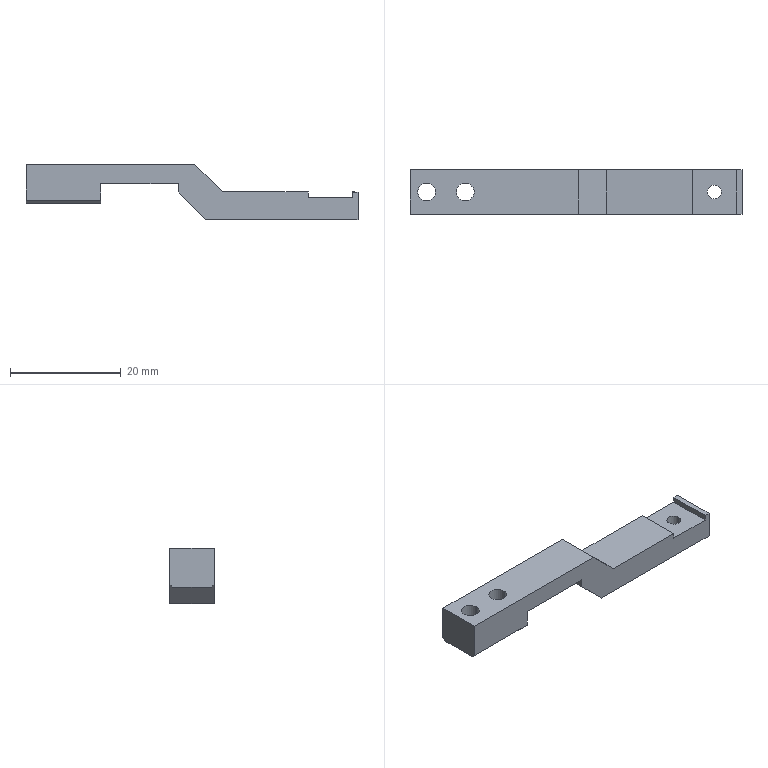Part | SolidWorks | features ICE 4, Chamfer 2, HoleWzd 2, Extrusion 1 | 1 solid | 25 faces | box 60 x 8 x 10 mm | volume 2368 mm3 | plane 19 | cylinder 6 | commonest cylinder face diameters 3.2 x4 2.5 x2
STEP:
#1=CARTESIAN_POINT('',(23.75,0.,-6.5));
#2=VERTEX_POINT('',#1);
#3=CARTESIAN_POINT('',(26.25,0.,-6.5));
#4=VERTEX_POINT('',#3);
#5=CARTESIAN_POINT('',(25.,0.,-6.5));
#6=DIRECTION('',(0.,0.,1.));
#7=DIRECTION('',(1.,0.,0.));
#8=AXIS2_PLACEMENT_3D('',#5,#6,#7);
#9=CIRCLE('',#8,1.25);
#10=EDGE_CURVE('',#2,#4,#9,.T.);
#11=ORIENTED_EDGE('',*,*,#10,.F.);
#12=CARTESIAN_POINT('',(23.75,0.,-2.5));
#13=VERTEX_POINT('',#12);
#14=CARTESIAN_POINT('',(23.75,0.,-2.5));
#15=DIRECTION('',(0.,0.,1.));
#16=VECTOR('',#15,1000.);
#17=LINE('',#14,#16);
#18=EDGE_CURVE('',#2,#13,#17,.T.);
#19=ORIENTED_EDGE('',*,*,#18,.T.);
#20=CARTESIAN_POINT('',(26.25,0.,-2.5));
#21=VERTEX_POINT('',#20);
#22=CARTESIAN_POINT('',(25.,0.,-2.5));
#23=DIRECTION('',(0.,0.,1.));
#24=DIRECTION('',(1.,0.,0.));
#25=AXIS2_PLACEMENT_3D('',#22,#23,#24);
#26=CIRCLE('',#25,1.25);
#27=EDGE_CURVE('',#13,#21,#26,.T.);
#28=ORIENTED_EDGE('',*,*,#27,.T.);
#29=CARTESIAN_POINT('',(26.25,0.,-2.5));
#30=DIRECTION('',(0.,0.,1.));
#31=VECTOR('',#30,1000.);
#32=LINE('',#29,#31);
#33=EDGE_CURVE('',#4,#21,#32,.T.);
#34=ORIENTED_EDGE('',*,*,#33,.F.);
#35=EDGE_LOOP('',(#11,#19,#28,#34));
#36=FACE_OUTER_BOUND('',#35,.T.);
#37=CARTESIAN_POINT('',(25.,0.,-2.5));
#38=DIRECTION('',(0.,0.,1.));
#39=DIRECTION('',(1.,0.,0.));
#40=AXIS2_PLACEMENT_3D('',#37,#38,#39);
#41=CYLINDRICAL_SURFACE('',#40,1.25);
#42=ADVANCED_FACE('',(#36),#41,.F.);
#43=CARTESIAN_POINT('',(-28.6,0.,-3.5));
#44=VERTEX_POINT('',#43);
#45=CARTESIAN_POINT('',(-25.4,0.,-3.5));
#46=VERTEX_POINT('',#45);
#47=CARTESIAN_POINT('',(-27.,0.,-3.5));
#48=DIRECTION('',(0.,0.,1.));
#49=DIRECTION('',(1.,0.,0.));
#50=AXIS2_PLACEMENT_3D('',#47,#48,#49);
#51=CIRCLE('',#50,1.6);
#52=EDGE_CURVE('',#44,#46,#51,.T.);
#53=ORIENTED_EDGE('',*,*,#52,.F.);
#54=CARTESIAN_POINT('',(-28.6,0.,3.5));
#55=VERTEX_POINT('',#54);
#56=CARTESIAN_POINT('',(-28.6,0.,3.5));
#57=DIRECTION('',(0.,0.,1.));
#58=VECTOR('',#57,1000.);
#59=LINE('',#56,#58);
#60=EDGE_CURVE('',#44,#55,#59,.T.);
#61=ORIENTED_EDGE('',*,*,#60,.T.);
#62=CARTESIAN_POINT('',(-25.4,0.,3.5));
#63=VERTEX_POINT('',#62);
#64=CARTESIAN_POINT('',(-27.,0.,3.5));
#65=DIRECTION('',(0.,0.,1.));
#66=DIRECTION('',(1.,0.,0.));
#67=AXIS2_PLACEMENT_3D('',#64,#65,#66);
#68=CIRCLE('',#67,1.6);
#69=EDGE_CURVE('',#55,#63,#68,.T.);
#70=ORIENTED_EDGE('',*,*,#69,.T.);
#71=CARTESIAN_POINT('',(-25.4,0.,3.5));
#72=DIRECTION('',(0.,0.,1.));
#73=VECTOR('',#72,1000.);
#74=LINE('',#71,#73);
#75=EDGE_CURVE('',#46,#63,#74,.T.);
#76=ORIENTED_EDGE('',*,*,#75,.F.);
#77=EDGE_LOOP('',(#53,#61,#70,#76));
#78=FACE_OUTER_BOUND('',#77,.T.);
#79=CARTESIAN_POINT('',(-27.,0.,3.5));
#80=DIRECTION('',(0.,0.,1.));
#81=DIRECTION('',(1.,0.,0.));
#82=AXIS2_PLACEMENT_3D('',#79,#80,#81);
#83=CYLINDRICAL_SURFACE('',#82,1.6);
#84=ADVANCED_FACE('',(#78),#83,.F.);
#85=CARTESIAN_POINT('',(-21.6,0.,-3.5));
#86=VERTEX_POINT('',#85);
#87=CARTESIAN_POINT('',(-18.4,0.,-3.5));
#88=VERTEX_POINT('',#87);
#89=CARTESIAN_POINT('',(-20.,0.,-3.5));
#90=DIRECTION('',(0.,0.,1.));
#91=DIRECTION('',(1.,0.,0.));
#92=AXIS2_PLACEMENT_3D('',#89,#90,#91);
#93=CIRCLE('',#92,1.6);
#94=EDGE_CURVE('',#86,#88,#93,.T.);
#95=ORIENTED_EDGE('',*,*,#94,.F.);
#96=CARTESIAN_POINT('',(-21.6,0.,3.5));
#97=VERTEX_POINT('',#96);
#98=CARTESIAN_POINT('',(-21.6,0.,3.5));
#99=DIRECTION('',(0.,0.,1.));
#100=VECTOR('',#99,1000.);
#101=LINE('',#98,#100);
#102=EDGE_CURVE('',#86,#97,#101,.T.);
#103=ORIENTED_EDGE('',*,*,#102,.T.);
#104=CARTESIAN_POINT('',(-18.4,0.,3.5));
#105=VERTEX_POINT('',#104);
#106=CARTESIAN_POINT('',(-20.,0.,3.5));
#107=DIRECTION('',(0.,0.,1.));
#108=DIRECTION('',(1.,0.,0.));
#109=AXIS2_PLACEMENT_3D('',#106,#107,#108);
#110=CIRCLE('',#109,1.6);
#111=EDGE_CURVE('',#97,#105,#110,.T.);
#112=ORIENTED_EDGE('',*,*,#111,.T.);
#113=CARTESIAN_POINT('',(-18.4,0.,3.5));
#114=DIRECTION('',(0.,0.,1.));
#115=VECTOR('',#114,1000.);
#116=LINE('',#113,#115);
#117=EDGE_CURVE('',#88,#105,#116,.T.);
#118=ORIENTED_EDGE('',*,*,#117,.F.);
#119=EDGE_LOOP('',(#95,#103,#112,#118));
#120=FACE_OUTER_BOUND('',#119,.T.);
#121=CARTESIAN_POINT('',(-20.,0.,3.5));
#122=DIRECTION('',(0.,0.,1.));
#123=DIRECTION('',(1.,0.,0.));
#124=AXIS2_PLACEMENT_3D('',#121,#122,#123);
#125=CYLINDRICAL_SURFACE('',#124,1.6);
#126=ADVANCED_FACE('',(#120),#125,.F.);
#127=CARTESIAN_POINT('',(21.,-4.,-1.5));
#128=VERTEX_POINT('',#127);
#129=CARTESIAN_POINT('',(5.5,-4.,-1.5));
#130=VERTEX_POINT('',#129);
#131=CARTESIAN_POINT('',(30.,-4.,-1.5));
#132=DIRECTION('',(-1.,0.,0.));
#133=VECTOR('',#132,1000.);
#134=LINE('',#131,#133);
#135=EDGE_CURVE('',#128,#130,#134,.T.);
#136=ORIENTED_EDGE('',*,*,#135,.F.);
#137=CARTESIAN_POINT('',(21.,4.,-1.5));
#138=VERTEX_POINT('',#137);
#139=CARTESIAN_POINT('',(21.,-4.,-1.5));
#140=DIRECTION('',(0.,-1.,0.));
#141=VECTOR('',#140,1000.);
#142=LINE('',#139,#141);
#143=EDGE_CURVE('',#138,#128,#142,.T.);
#144=ORIENTED_EDGE('',*,*,#143,.F.);
#145=CARTESIAN_POINT('',(5.5,4.,-1.5));
#146=VERTEX_POINT('',#145);
#147=CARTESIAN_POINT('',(30.,4.,-1.5));
#148=DIRECTION('',(-1.,0.,0.));
#149=VECTOR('',#148,1000.);
#150=LINE('',#147,#149);
#151=EDGE_CURVE('',#138,#146,#150,.T.);
#152=ORIENTED_EDGE('',*,*,#151,.T.);
#153=CARTESIAN_POINT('',(5.5,-4.,-1.5));
#154=DIRECTION('',(0.,1.,0.));
#155=VECTOR('',#154,1000.);
#156=LINE('',#153,#155);
#157=EDGE_CURVE('',#130,#146,#156,.T.);
#158=ORIENTED_EDGE('',*,*,#157,.F.);
#159=EDGE_LOOP('',(#136,#144,#152,#158));
#160=FACE_OUTER_BOUND('',#159,.T.);
#161=CARTESIAN_POINT('',(30.,-4.,-1.5));
#162=DIRECTION('',(0.,0.,-1.));
#163=DIRECTION('',(-1.,0.,0.));
#164=AXIS2_PLACEMENT_3D('',#161,#162,#163);
#165=PLANE('',#164);
#166=ADVANCED_FACE('',(#160),#165,.F.);
#167=CARTESIAN_POINT('',(-27.,0.,-3.5));
#168=DIRECTION('',(0.,0.,1.));
#169=DIRECTION('',(1.,0.,0.));
#170=AXIS2_PLACEMENT_3D('',#167,#168,#169);
#171=CIRCLE('',#170,1.6);
#172=EDGE_CURVE('',#46,#44,#171,.T.);
#173=ORIENTED_EDGE('',*,*,#172,.T.);
#174=ORIENTED_EDGE('',*,*,#52,.T.);
#175=EDGE_LOOP('',(#173,#174));
#176=FACE_BOUND('',#175,.T.);
#177=CARTESIAN_POINT('',(-20.,0.,-3.5));
#178=DIRECTION('',(0.,0.,1.));
#179=DIRECTION('',(1.,0.,0.));
#180=AXIS2_PLACEMENT_3D('',#177,#178,#179);
#181=CIRCLE('',#180,1.6);
#182=EDGE_CURVE('',#88,#86,#181,.T.);
#183=ORIENTED_EDGE('',*,*,#182,.T.);
#184=ORIENTED_EDGE('',*,*,#94,.T.);
#185=EDGE_LOOP('',(#183,#184));
#186=FACE_BOUND('',#185,.T.);
#187=CARTESIAN_POINT('',(-16.5,-3.5,-3.5));
#188=VERTEX_POINT('',#187);
#189=CARTESIAN_POINT('',(-16.5,3.5,-3.5));
#190=VERTEX_POINT('',#189);
#191=CARTESIAN_POINT('',(-16.5,-4.,-3.5));
#192=DIRECTION('',(0.,1.,0.));
#193=VECTOR('',#192,1000.);
#194=LINE('',#191,#193);
#195=EDGE_CURVE('',#188,#190,#194,.T.);
#196=ORIENTED_EDGE('',*,*,#195,.F.);
#197=CARTESIAN_POINT('',(-30.,-3.5,-3.5));
#198=VERTEX_POINT('',#197);
#199=CARTESIAN_POINT('',(0.,-3.5,-3.5));
#200=DIRECTION('',(-1.,0.,0.));
#201=VECTOR('',#200,1000.);
#202=LINE('',#199,#201);
#203=EDGE_CURVE('',#188,#198,#202,.T.);
#204=ORIENTED_EDGE('',*,*,#203,.T.);
#205=CARTESIAN_POINT('',(-30.,3.5,-3.5));
#206=VERTEX_POINT('',#205);
#207=CARTESIAN_POINT('',(-30.,4.,-3.5));
#208=DIRECTION('',(0.,-1.,0.));
#209=VECTOR('',#208,1000.);
#210=LINE('',#207,#209);
#211=EDGE_CURVE('',#206,#198,#210,.T.);
#212=ORIENTED_EDGE('',*,*,#211,.F.);
#213=CARTESIAN_POINT('',(0.,3.5,-3.5));
#214=DIRECTION('',(1.,0.,0.));
#215=VECTOR('',#214,1000.);
#216=LINE('',#213,#215);
#217=EDGE_CURVE('',#206,#190,#216,.T.);
#218=ORIENTED_EDGE('',*,*,#217,.T.);
#219=EDGE_LOOP('',(#196,#204,#212,#218));
#220=FACE_OUTER_BOUND('',#219,.T.);
#221=CARTESIAN_POINT('',(0.,0.,-3.5));
#222=DIRECTION('',(0.,0.,1.));
#223=DIRECTION('',(1.,0.,0.));
#224=AXIS2_PLACEMENT_3D('',#221,#222,#223);
#225=PLANE('',#224);
#226=ADVANCED_FACE('',(#176,#186,#220),#225,.F.);
#227=CARTESIAN_POINT('',(30.,4.,-1.5));
#228=VERTEX_POINT('',#227);
#229=CARTESIAN_POINT('',(30.,4.,-6.5));
#230=VERTEX_POINT('',#229);
#231=CARTESIAN_POINT('',(30.,4.,3.5));
#232=DIRECTION('',(0.,0.,-1.));
#233=VECTOR('',#232,1000.);
#234=LINE('',#231,#233);
#235=EDGE_CURVE('',#228,#230,#234,.T.);
#236=ORIENTED_EDGE('',*,*,#235,.F.);
#237=CARTESIAN_POINT('',(30.,-4.,-1.5));
#238=VERTEX_POINT('',#237);
#239=CARTESIAN_POINT('',(30.,-4.,-1.5));
#240=DIRECTION('',(0.,1.,0.));
#241=VECTOR('',#240,1000.);
#242=LINE('',#239,#241);
#243=EDGE_CURVE('',#238,#228,#242,.T.);
#244=ORIENTED_EDGE('',*,*,#243,.F.);
#245=CARTESIAN_POINT('',(30.,-4.,-6.5));
#246=VERTEX_POINT('',#245);
#247=CARTESIAN_POINT('',(30.,-4.,3.5));
#248=DIRECTION('',(0.,0.,-1.));
#249=VECTOR('',#248,1000.);
#250=LINE('',#247,#249);
#251=EDGE_CURVE('',#238,#246,#250,.T.);
#252=ORIENTED_EDGE('',*,*,#251,.T.);
#253=CARTESIAN_POINT('',(30.,4.,-6.5));
#254=DIRECTION('',(0.,-1.,0.));
#255=VECTOR('',#254,1000.);
#256=LINE('',#253,#255);
#257=EDGE_CURVE('',#230,#246,#256,.T.);
#258=ORIENTED_EDGE('',*,*,#257,.F.);
#259=EDGE_LOOP('',(#236,#244,#252,#258));
#260=FACE_OUTER_BOUND('',#259,.T.);
#261=CARTESIAN_POINT('',(30.,4.,3.5));
#262=DIRECTION('',(-1.,0.,0.));
#263=DIRECTION('',(0.,0.,1.));
#264=AXIS2_PLACEMENT_3D('',#261,#262,#263);
#265=PLANE('',#264);
#266=ADVANCED_FACE('',(#260),#265,.F.);
#267=CARTESIAN_POINT('',(-16.5,4.,-3.));
#268=VERTEX_POINT('',#267);
#269=CARTESIAN_POINT('',(-16.5,4.,0.));
#270=VERTEX_POINT('',#269);
#271=CARTESIAN_POINT('',(-16.5,4.,-3.5));
#272=DIRECTION('',(0.,0.,1.));
#273=VECTOR('',#272,1000.);
#274=LINE('',#271,#273);
#275=EDGE_CURVE('',#268,#270,#274,.T.);
#276=ORIENTED_EDGE('',*,*,#275,.F.);
#277=CARTESIAN_POINT('',(-30.,4.,-3.));
#278=VERTEX_POINT('',#277);
#279=CARTESIAN_POINT('',(-30.,4.,-3.));
#280=DIRECTION('',(-1.,0.,0.));
#281=VECTOR('',#280,1000.);
#282=LINE('',#279,#281);
#283=EDGE_CURVE('',#268,#278,#282,.T.);
#284=ORIENTED_EDGE('',*,*,#283,.T.);
#285=CARTESIAN_POINT('',(-30.,4.,3.5));
#286=VERTEX_POINT('',#285);
#287=CARTESIAN_POINT('',(-30.,4.,3.5));
#288=DIRECTION('',(0.,0.,-1.));
#289=VECTOR('',#288,1000.);
#290=LINE('',#287,#289);
#291=EDGE_CURVE('',#286,#278,#290,.T.);
#292=ORIENTED_EDGE('',*,*,#291,.F.);
#293=CARTESIAN_POINT('',(0.5,4.,3.5));
#294=VERTEX_POINT('',#293);
#295=CARTESIAN_POINT('',(-30.,4.,3.5));
#296=DIRECTION('',(-1.,0.,0.));
#297=VECTOR('',#296,1000.);
#298=LINE('',#295,#297);
#299=EDGE_CURVE('',#294,#286,#298,.T.);
#300=ORIENTED_EDGE('',*,*,#299,.F.);
#301=CARTESIAN_POINT('',(0.5,4.,3.5));
#302=DIRECTION('',(0.7071,0.,-0.7071));
#303=VECTOR('',#302,1000.);
#304=LINE('',#301,#303);
#305=EDGE_CURVE('',#294,#146,#304,.T.);
#306=ORIENTED_EDGE('',*,*,#305,.T.);
#307=ORIENTED_EDGE('',*,*,#151,.F.);
#308=CARTESIAN_POINT('',(21.,4.,-2.5));
#309=VERTEX_POINT('',#308);
#310=CARTESIAN_POINT('',(21.,4.,-2.5));
#311=DIRECTION('',(0.,0.,1.));
#312=VECTOR('',#311,1000.);
#313=LINE('',#310,#312);
#314=EDGE_CURVE('',#309,#138,#313,.T.);
#315=ORIENTED_EDGE('',*,*,#314,.F.);
#316=CARTESIAN_POINT('',(29.,4.,-2.5));
#317=VERTEX_POINT('',#316);
#318=CARTESIAN_POINT('',(21.,4.,-2.5));
#319=DIRECTION('',(-1.,0.,0.));
#320=VECTOR('',#319,1000.);
#321=LINE('',#318,#320);
#322=EDGE_CURVE('',#317,#309,#321,.T.);
#323=ORIENTED_EDGE('',*,*,#322,.F.);
#324=CARTESIAN_POINT('',(29.,4.,-1.5));
#325=VERTEX_POINT('',#324);
#326=CARTESIAN_POINT('',(29.,4.,-2.5));
#327=DIRECTION('',(0.,0.,1.));
#328=VECTOR('',#327,1000.);
#329=LINE('',#326,#328);
#330=EDGE_CURVE('',#317,#325,#329,.T.);
#331=ORIENTED_EDGE('',*,*,#330,.T.);
#332=CARTESIAN_POINT('',(30.,4.,-1.5));
#333=DIRECTION('',(-1.,0.,0.));
#334=VECTOR('',#333,1000.);
#335=LINE('',#332,#334);
#336=EDGE_CURVE('',#228,#325,#335,.T.);
#337=ORIENTED_EDGE('',*,*,#336,.F.);
#338=ORIENTED_EDGE('',*,*,#235,.T.);
#339=CARTESIAN_POINT('',(2.5,4.,-6.5));
#340=VERTEX_POINT('',#339);
#341=CARTESIAN_POINT('',(-2.5,4.,-6.5));
#342=DIRECTION('',(1.,0.,0.));
#343=VECTOR('',#342,1000.);
#344=LINE('',#341,#343);
#345=EDGE_CURVE('',#340,#230,#344,.T.);
#346=ORIENTED_EDGE('',*,*,#345,.F.);
#347=CARTESIAN_POINT('',(-2.5,4.,-1.5));
#348=VERTEX_POINT('',#347);
#349=CARTESIAN_POINT('',(2.5,4.,-6.5));
#350=DIRECTION('',(-0.7071,0.,0.7071));
#351=VECTOR('',#350,1000.);
#352=LINE('',#349,#351);
#353=EDGE_CURVE('',#340,#348,#352,.T.);
#354=ORIENTED_EDGE('',*,*,#353,.T.);
#355=CARTESIAN_POINT('',(-2.5,4.,0.));
#356=VERTEX_POINT('',#355);
#357=CARTESIAN_POINT('',(-2.5,4.,-3.5));
#358=DIRECTION('',(0.,0.,-1.));
#359=VECTOR('',#358,1000.);
#360=LINE('',#357,#359);
#361=EDGE_CURVE('',#356,#348,#360,.T.);
#362=ORIENTED_EDGE('',*,*,#361,.F.);
#363=CARTESIAN_POINT('',(-16.5,4.,0.));
#364=DIRECTION('',(1.,0.,0.));
#365=VECTOR('',#364,1000.);
#366=LINE('',#363,#365);
#367=EDGE_CURVE('',#270,#356,#366,.T.);
#368=ORIENTED_EDGE('',*,*,#367,.F.);
#369=EDGE_LOOP('',(#276,#284,#292,#300,#306,#307,#315,#323,#331,#337,#338,#346,#354,#362,#368));
#370=FACE_OUTER_BOUND('',#369,.T.);
#371=CARTESIAN_POINT('',(-30.,4.,3.5));
#372=DIRECTION('',(0.,-1.,0.));
#373=DIRECTION('',(0.,0.,-1.));
#374=AXIS2_PLACEMENT_3D('',#371,#372,#373);
#375=PLANE('',#374);
#376=ADVANCED_FACE('',(#370),#375,.F.);
#377=ORIENTED_EDGE('',*,*,#211,.T.);
#378=CARTESIAN_POINT('',(-30.,-4.,-3.));
#379=VERTEX_POINT('',#378);
#380=CARTESIAN_POINT('',(-30.,-4.,-3.));
#381=DIRECTION('',(0.,-0.7071,0.7071));
#382=VECTOR('',#381,1000.);
#383=LINE('',#380,#382);
#384=EDGE_CURVE('',#198,#379,#383,.T.);
#385=ORIENTED_EDGE('',*,*,#384,.T.);
#386=CARTESIAN_POINT('',(-30.,-4.,3.5));
#387=VERTEX_POINT('',#386);
#388=CARTESIAN_POINT('',(-30.,-4.,3.5));
#389=DIRECTION('',(0.,0.,-1.));
#390=VECTOR('',#389,1000.);
#391=LINE('',#388,#390);
#392=EDGE_CURVE('',#387,#379,#391,.T.);
#393=ORIENTED_EDGE('',*,*,#392,.F.);
#394=CARTESIAN_POINT('',(-30.,4.,3.5));
#395=DIRECTION('',(0.,-1.,0.));
#396=VECTOR('',#395,1000.);
#397=LINE('',#394,#396);
#398=EDGE_CURVE('',#286,#387,#397,.T.);
#399=ORIENTED_EDGE('',*,*,#398,.F.);
#400=ORIENTED_EDGE('',*,*,#291,.T.);
#401=CARTESIAN_POINT('',(-30.,4.,-3.));
#402=DIRECTION('',(0.,-0.7071,-0.7071));
#403=VECTOR('',#402,1000.);
#404=LINE('',#401,#403);
#405=EDGE_CURVE('',#278,#206,#404,.T.);
#406=ORIENTED_EDGE('',*,*,#405,.T.);
#407=EDGE_LOOP('',(#377,#385,#393,#399,#400,#406));
#408=FACE_OUTER_BOUND('',#407,.T.);
#409=CARTESIAN_POINT('',(-30.,4.,3.5));
#410=DIRECTION('',(1.,0.,0.));
#411=DIRECTION('',(0.,0.,-1.));
#412=AXIS2_PLACEMENT_3D('',#409,#410,#411);
#413=PLANE('',#412);
#414=ADVANCED_FACE('',(#408),#413,.F.);
#415=ORIENTED_EDGE('',*,*,#392,.T.);
#416=CARTESIAN_POINT('',(-16.5,-4.,-3.));
#417=VERTEX_POINT('',#416);
#418=CARTESIAN_POINT('',(-30.,-4.,-3.));
#419=DIRECTION('',(1.,0.,0.));
#420=VECTOR('',#419,1000.);
#421=LINE('',#418,#420);
#422=EDGE_CURVE('',#379,#417,#421,.T.);
#423=ORIENTED_EDGE('',*,*,#422,.T.);
#424=CARTESIAN_POINT('',(-16.5,-4.,0.));
#425=VERTEX_POINT('',#424);
#426=CARTESIAN_POINT('',(-16.5,-4.,-3.5));
#427=DIRECTION('',(0.,0.,1.));
#428=VECTOR('',#427,1000.);
#429=LINE('',#426,#428);
#430=EDGE_CURVE('',#417,#425,#429,.T.);
#431=ORIENTED_EDGE('',*,*,#430,.T.);
#432=CARTESIAN_POINT('',(-2.5,-4.,0.));
#433=VERTEX_POINT('',#432);
#434=CARTESIAN_POINT('',(-16.5,-4.,0.));
#435=DIRECTION('',(1.,0.,0.));
#436=VECTOR('',#435,1000.);
#437=LINE('',#434,#436);
#438=EDGE_CURVE('',#425,#433,#437,.T.);
#439=ORIENTED_EDGE('',*,*,#438,.T.);
#440=CARTESIAN_POINT('',(-2.5,-4.,-1.5));
#441=VERTEX_POINT('',#440);
#442=CARTESIAN_POINT('',(-2.5,-4.,-3.5));
#443=DIRECTION('',(0.,0.,-1.));
#444=VECTOR('',#443,1000.);
#445=LINE('',#442,#444);
#446=EDGE_CURVE('',#433,#441,#445,.T.);
#447=ORIENTED_EDGE('',*,*,#446,.T.);
#448=CARTESIAN_POINT('',(2.5,-4.,-6.5));
#449=VERTEX_POINT('',#448);
#450=CARTESIAN_POINT('',(2.5,-4.,-6.5));
#451=DIRECTION('',(0.7071,0.,-0.7071));
#452=VECTOR('',#451,1000.);
#453=LINE('',#450,#452);
#454=EDGE_CURVE('',#441,#449,#453,.T.);
#455=ORIENTED_EDGE('',*,*,#454,.T.);
#456=CARTESIAN_POINT('',(30.,-4.,-6.5));
#457=DIRECTION('',(-1.,0.,0.));
#458=VECTOR('',#457,1000.);
#459=LINE('',#456,#458);
#460=EDGE_CURVE('',#246,#449,#459,.T.);
#461=ORIENTED_EDGE('',*,*,#460,.F.);
#462=ORIENTED_EDGE('',*,*,#251,.F.);
#463=CARTESIAN_POINT('',(29.,-4.,-1.5));
#464=VERTEX_POINT('',#463);
#465=CARTESIAN_POINT('',(30.,-4.,-1.5));
#466=DIRECTION('',(-1.,0.,0.));
#467=VECTOR('',#466,1000.);
#468=LINE('',#465,#467);
#469=EDGE_CURVE('',#238,#464,#468,.T.);
#470=ORIENTED_EDGE('',*,*,#469,.T.);
#471=CARTESIAN_POINT('',(29.,-4.,-2.5));
#472=VERTEX_POINT('',#471);
#473=CARTESIAN_POINT('',(29.,-4.,-2.5));
#474=DIRECTION('',(0.,0.,1.));
#475=VECTOR('',#474,1000.);
#476=LINE('',#473,#475);
#477=EDGE_CURVE('',#472,#464,#476,.T.);
#478=ORIENTED_EDGE('',*,*,#477,.F.);
#479=CARTESIAN_POINT('',(21.,-4.,-2.5));
#480=VERTEX_POINT('',#479);
#481=CARTESIAN_POINT('',(21.,-4.,-2.5));
#482=DIRECTION('',(1.,0.,0.));
#483=VECTOR('',#482,1000.);
#484=LINE('',#481,#483);
#485=EDGE_CURVE('',#480,#472,#484,.T.);
#486=ORIENTED_EDGE('',*,*,#485,.F.);
#487=CARTESIAN_POINT('',(21.,-4.,-2.5));
#488=DIRECTION('',(0.,0.,1.));
#489=VECTOR('',#488,1000.);
#490=LINE('',#487,#489);
#491=EDGE_CURVE('',#480,#128,#490,.T.);
#492=ORIENTED_EDGE('',*,*,#491,.T.);
#493=ORIENTED_EDGE('',*,*,#135,.T.);
#494=CARTESIAN_POINT('',(0.5,-4.,3.5));
#495=VERTEX_POINT('',#494);
#496=CARTESIAN_POINT('',(0.5,-4.,3.5));
#497=DIRECTION('',(-0.7071,0.,0.7071));
#498=VECTOR('',#497,1000.);
#499=LINE('',#496,#498);
#500=EDGE_CURVE('',#130,#495,#499,.T.);
#501=ORIENTED_EDGE('',*,*,#500,.T.);
#502=CARTESIAN_POINT('',(-30.,-4.,3.5));
#503=DIRECTION('',(1.,0.,0.));
#504=VECTOR('',#503,1000.);
#505=LINE('',#502,#504);
#506=EDGE_CURVE('',#387,#495,#505,.T.);
#507=ORIENTED_EDGE('',*,*,#506,.F.);
#508=EDGE_LOOP('',(#415,#423,#431,#439,#447,#455,#461,#462,#470,#478,#486,#492,#493,#501,#507));
#509=FACE_OUTER_BOUND('',#508,.T.);
#510=CARTESIAN_POINT('',(-30.,-4.,3.5));
#511=DIRECTION('',(0.,1.,0.));
#512=DIRECTION('',(0.,0.,1.));
#513=AXIS2_PLACEMENT_3D('',#510,#511,#512);
#514=PLANE('',#513);
#515=ADVANCED_FACE('',(#509),#514,.F.);
#516=CARTESIAN_POINT('',(-27.,0.,3.5));
#517=DIRECTION('',(0.,0.,1.));
#518=DIRECTION('',(1.,0.,0.));
#519=AXIS2_PLACEMENT_3D('',#516,#517,#518);
#520=CIRCLE('',#519,1.6);
#521=EDGE_CURVE('',#63,#55,#520,.T.);
#522=ORIENTED_EDGE('',*,*,#521,.F.);
#523=ORIENTED_EDGE('',*,*,#69,.F.);
#524=EDGE_LOOP('',(#522,#523));
#525=FACE_BOUND('',#524,.T.);
#526=CARTESIAN_POINT('',(-20.,0.,3.5));
#527=DIRECTION('',(0.,0.,1.));
#528=DIRECTION('',(1.,0.,0.));
#529=AXIS2_PLACEMENT_3D('',#526,#527,#528);
#530=CIRCLE('',#529,1.6);
#531=EDGE_CURVE('',#105,#97,#530,.T.);
#532=ORIENTED_EDGE('',*,*,#531,.F.);
#533=ORIENTED_EDGE('',*,*,#111,.F.);
#534=EDGE_LOOP('',(#532,#533));
#535=FACE_BOUND('',#534,.T.);
#536=ORIENTED_EDGE('',*,*,#506,.T.);
#537=CARTESIAN_POINT('',(0.5,4.,3.5));
#538=DIRECTION('',(0.,1.,0.));
#539=VECTOR('',#538,1000.);
#540=LINE('',#537,#539);
#541=EDGE_CURVE('',#495,#294,#540,.T.);
#542=ORIENTED_EDGE('',*,*,#541,.T.);
#543=ORIENTED_EDGE('',*,*,#299,.T.);
#544=ORIENTED_EDGE('',*,*,#398,.T.);
#545=EDGE_LOOP('',(#536,#542,#543,#544));
#546=FACE_OUTER_BOUND('',#545,.T.);
#547=CARTESIAN_POINT('',(0.,0.,3.5));
#548=DIRECTION('',(0.,0.,1.));
#549=DIRECTION('',(1.,0.,0.));
#550=AXIS2_PLACEMENT_3D('',#547,#548,#549);
#551=PLANE('',#550);
#552=ADVANCED_FACE('',(#525,#535,#546),#551,.T.);
#553=ORIENTED_EDGE('',*,*,#430,.F.);
#554=CARTESIAN_POINT('',(-16.5,-4.,-3.));
#555=DIRECTION('',(0.,0.7071,-0.7071));
#556=VECTOR('',#555,1000.);
#557=LINE('',#554,#556);
#558=EDGE_CURVE('',#417,#188,#557,.T.);
#559=ORIENTED_EDGE('',*,*,#558,.T.);
#560=ORIENTED_EDGE('',*,*,#195,.T.);
#561=CARTESIAN_POINT('',(-16.5,4.,-3.));
#562=DIRECTION('',(0.,0.7071,0.7071));
#563=VECTOR('',#562,1000.);
#564=LINE('',#561,#563);
#565=EDGE_CURVE('',#190,#268,#564,.T.);
#566=ORIENTED_EDGE('',*,*,#565,.T.);
#567=ORIENTED_EDGE('',*,*,#275,.T.);
#568=CARTESIAN_POINT('',(-16.5,-4.,0.));
#569=DIRECTION('',(0.,1.,0.));
#570=VECTOR('',#569,1000.);
#571=LINE('',#568,#570);
#572=EDGE_CURVE('',#425,#270,#571,.T.);
#573=ORIENTED_EDGE('',*,*,#572,.F.);
#574=EDGE_LOOP('',(#553,#559,#560,#566,#567,#573));
#575=FACE_OUTER_BOUND('',#574,.T.);
#576=CARTESIAN_POINT('',(-16.5,-4.,-3.5));
#577=DIRECTION('',(-1.,0.,0.));
#578=DIRECTION('',(0.,0.,1.));
#579=AXIS2_PLACEMENT_3D('',#576,#577,#578);
#580=PLANE('',#579);
#581=ADVANCED_FACE('',(#575),#580,.F.);
#582=ORIENTED_EDGE('',*,*,#361,.T.);
#583=CARTESIAN_POINT('',(-2.5,-4.,-1.5));
#584=DIRECTION('',(0.,-1.,0.));
#585=VECTOR('',#584,1000.);
#586=LINE('',#583,#585);
#587=EDGE_CURVE('',#348,#441,#586,.T.);
#588=ORIENTED_EDGE('',*,*,#587,.T.);
#589=ORIENTED_EDGE('',*,*,#446,.F.);
#590=CARTESIAN_POINT('',(-2.5,-4.,0.));
#591=DIRECTION('',(0.,1.,0.));
#592=VECTOR('',#591,1000.);
#593=LINE('',#590,#592);
#594=EDGE_CURVE('',#433,#356,#593,.T.);
#595=ORIENTED_EDGE('',*,*,#594,.T.);
#596=EDGE_LOOP('',(#582,#588,#589,#595));
#597=FACE_OUTER_BOUND('',#596,.T.);
#598=CARTESIAN_POINT('',(-2.5,-4.,-3.5));
#599=DIRECTION('',(1.,0.,0.));
#600=DIRECTION('',(0.,0.,-1.));
#601=AXIS2_PLACEMENT_3D('',#598,#599,#600);
#602=PLANE('',#601);
#603=ADVANCED_FACE('',(#597),#602,.F.);
#604=ORIENTED_EDGE('',*,*,#367,.T.);
#605=ORIENTED_EDGE('',*,*,#594,.F.);
#606=ORIENTED_EDGE('',*,*,#438,.F.);
#607=ORIENTED_EDGE('',*,*,#572,.T.);
#608=EDGE_LOOP('',(#604,#605,#606,#607));
#609=FACE_OUTER_BOUND('',#608,.T.);
#610=CARTESIAN_POINT('',(-16.5,-4.,0.));
#611=DIRECTION('',(0.,0.,1.));
#612=DIRECTION('',(1.,0.,0.));
#613=AXIS2_PLACEMENT_3D('',#610,#611,#612);
#614=PLANE('',#613);
#615=ADVANCED_FACE('',(#609),#614,.F.);
#616=CARTESIAN_POINT('',(25.,0.,-6.5));
#617=DIRECTION('',(0.,0.,1.));
#618=DIRECTION('',(1.,0.,0.));
#619=AXIS2_PLACEMENT_3D('',#616,#617,#618);
#620=CIRCLE('',#619,1.25);
#621=EDGE_CURVE('',#4,#2,#620,.T.);
#622=ORIENTED_EDGE('',*,*,#621,.T.);
#623=ORIENTED_EDGE('',*,*,#10,.T.);
#624=EDGE_LOOP('',(#622,#623));
#625=FACE_BOUND('',#624,.T.);
#626=ORIENTED_EDGE('',*,*,#460,.T.);
#627=CARTESIAN_POINT('',(2.5,4.,-6.5));
#628=DIRECTION('',(0.,1.,0.));
#629=VECTOR('',#628,1000.);
#630=LINE('',#627,#629);
#631=EDGE_CURVE('',#449,#340,#630,.T.);
#632=ORIENTED_EDGE('',*,*,#631,.T.);
#633=ORIENTED_EDGE('',*,*,#345,.T.);
#634=ORIENTED_EDGE('',*,*,#257,.T.);
#635=EDGE_LOOP('',(#626,#632,#633,#634));
#636=FACE_OUTER_BOUND('',#635,.T.);
#637=CARTESIAN_POINT('',(0.,0.,-6.5));
#638=DIRECTION('',(0.,0.,-1.));
#639=DIRECTION('',(-1.,0.,0.));
#640=AXIS2_PLACEMENT_3D('',#637,#638,#639);
#641=PLANE('',#640);
#642=ADVANCED_FACE('',(#625,#636),#641,.T.);
#643=ORIENTED_EDGE('',*,*,#336,.T.);
#644=CARTESIAN_POINT('',(29.,-4.,-1.5));
#645=DIRECTION('',(0.,1.,0.));
#646=VECTOR('',#645,1000.);
#647=LINE('',#644,#646);
#648=EDGE_CURVE('',#464,#325,#647,.T.);
#649=ORIENTED_EDGE('',*,*,#648,.F.);
#650=ORIENTED_EDGE('',*,*,#469,.F.);
#651=ORIENTED_EDGE('',*,*,#243,.T.);
#652=EDGE_LOOP('',(#643,#649,#650,#651));
#653=FACE_OUTER_BOUND('',#652,.T.);
#654=CARTESIAN_POINT('',(30.,-4.,-1.5));
#655=DIRECTION('',(0.,0.,-1.));
#656=DIRECTION('',(-1.,0.,0.));
#657=AXIS2_PLACEMENT_3D('',#654,#655,#656);
#658=PLANE('',#657);
#659=ADVANCED_FACE('',(#653),#658,.F.);
#660=ORIENTED_EDGE('',*,*,#454,.F.);
#661=ORIENTED_EDGE('',*,*,#587,.F.);
#662=ORIENTED_EDGE('',*,*,#353,.F.);
#663=ORIENTED_EDGE('',*,*,#631,.F.);
#664=EDGE_LOOP('',(#660,#661,#662,#663));
#665=FACE_OUTER_BOUND('',#664,.T.);
#666=CARTESIAN_POINT('',(2.5,0.,-6.5));
#667=DIRECTION('',(-0.7071,0.,-0.7071));
#668=DIRECTION('',(0.,-1.,0.));
#669=AXIS2_PLACEMENT_3D('',#666,#667,#668);
#670=PLANE('',#669);
#671=ADVANCED_FACE('',(#665),#670,.T.);
#672=ORIENTED_EDGE('',*,*,#500,.F.);
#673=ORIENTED_EDGE('',*,*,#157,.T.);
#674=ORIENTED_EDGE('',*,*,#305,.F.);
#675=ORIENTED_EDGE('',*,*,#541,.F.);
#676=EDGE_LOOP('',(#672,#673,#674,#675));
#677=FACE_OUTER_BOUND('',#676,.T.);
#678=CARTESIAN_POINT('',(0.5,0.,3.5));
#679=DIRECTION('',(0.7071,0.,0.7071));
#680=DIRECTION('',(0.,-1.,0.));
#681=AXIS2_PLACEMENT_3D('',#678,#679,#680);
#682=PLANE('',#681);
#683=ADVANCED_FACE('',(#677),#682,.T.);
#684=ORIENTED_EDGE('',*,*,#102,.F.);
#685=ORIENTED_EDGE('',*,*,#182,.F.);
#686=ORIENTED_EDGE('',*,*,#117,.T.);
#687=ORIENTED_EDGE('',*,*,#531,.T.);
#688=EDGE_LOOP('',(#684,#685,#686,#687));
#689=FACE_OUTER_BOUND('',#688,.T.);
#690=CARTESIAN_POINT('',(-20.,0.,3.5));
#691=DIRECTION('',(0.,0.,1.));
#692=DIRECTION('',(1.,0.,0.));
#693=AXIS2_PLACEMENT_3D('',#690,#691,#692);
#694=CYLINDRICAL_SURFACE('',#693,1.6);
#695=ADVANCED_FACE('',(#689),#694,.F.);
#696=ORIENTED_EDGE('',*,*,#60,.F.);
#697=ORIENTED_EDGE('',*,*,#172,.F.);
#698=ORIENTED_EDGE('',*,*,#75,.T.);
#699=ORIENTED_EDGE('',*,*,#521,.T.);
#700=EDGE_LOOP('',(#696,#697,#698,#699));
#701=FACE_OUTER_BOUND('',#700,.T.);
#702=CARTESIAN_POINT('',(-27.,0.,3.5));
#703=DIRECTION('',(0.,0.,1.));
#704=DIRECTION('',(1.,0.,0.));
#705=AXIS2_PLACEMENT_3D('',#702,#703,#704);
#706=CYLINDRICAL_SURFACE('',#705,1.6);
#707=ADVANCED_FACE('',(#701),#706,.F.);
#708=ORIENTED_EDGE('',*,*,#143,.T.);
#709=ORIENTED_EDGE('',*,*,#491,.F.);
#710=CARTESIAN_POINT('',(21.,-4.,-2.5));
#711=DIRECTION('',(0.,-1.,0.));
#712=VECTOR('',#711,1000.);
#713=LINE('',#710,#712);
#714=EDGE_CURVE('',#309,#480,#713,.T.);
#715=ORIENTED_EDGE('',*,*,#714,.F.);
#716=ORIENTED_EDGE('',*,*,#314,.T.);
#717=EDGE_LOOP('',(#708,#709,#715,#716));
#718=FACE_OUTER_BOUND('',#717,.T.);
#719=CARTESIAN_POINT('',(21.,-4.,-2.5));
#720=DIRECTION('',(-1.,0.,0.));
#721=DIRECTION('',(0.,0.,1.));
#722=AXIS2_PLACEMENT_3D('',#719,#720,#721);
#723=PLANE('',#722);
#724=ADVANCED_FACE('',(#718),#723,.F.);
#725=ORIENTED_EDGE('',*,*,#648,.T.);
#726=ORIENTED_EDGE('',*,*,#330,.F.);
#727=CARTESIAN_POINT('',(29.,-4.,-2.5));
#728=DIRECTION('',(0.,1.,0.));
#729=VECTOR('',#728,1000.);
#730=LINE('',#727,#729);
#731=EDGE_CURVE('',#472,#317,#730,.T.);
#732=ORIENTED_EDGE('',*,*,#731,.F.);
#733=ORIENTED_EDGE('',*,*,#477,.T.);
#734=EDGE_LOOP('',(#725,#726,#732,#733));
#735=FACE_OUTER_BOUND('',#734,.T.);
#736=CARTESIAN_POINT('',(29.,-4.,-2.5));
#737=DIRECTION('',(1.,0.,0.));
#738=DIRECTION('',(0.,0.,-1.));
#739=AXIS2_PLACEMENT_3D('',#736,#737,#738);
#740=PLANE('',#739);
#741=ADVANCED_FACE('',(#735),#740,.F.);
#742=CARTESIAN_POINT('',(25.,0.,-2.5));
#743=DIRECTION('',(0.,0.,1.));
#744=DIRECTION('',(1.,0.,0.));
#745=AXIS2_PLACEMENT_3D('',#742,#743,#744);
#746=CIRCLE('',#745,1.25);
#747=EDGE_CURVE('',#21,#13,#746,.T.);
#748=ORIENTED_EDGE('',*,*,#747,.F.);
#749=ORIENTED_EDGE('',*,*,#27,.F.);
#750=EDGE_LOOP('',(#748,#749));
#751=FACE_BOUND('',#750,.T.);
#752=ORIENTED_EDGE('',*,*,#714,.T.);
#753=ORIENTED_EDGE('',*,*,#485,.T.);
#754=ORIENTED_EDGE('',*,*,#731,.T.);
#755=ORIENTED_EDGE('',*,*,#322,.T.);
#756=EDGE_LOOP('',(#752,#753,#754,#755));
#757=FACE_OUTER_BOUND('',#756,.T.);
#758=CARTESIAN_POINT('',(0.,0.,-2.5));
#759=DIRECTION('',(0.,0.,-1.));
#760=DIRECTION('',(-1.,0.,0.));
#761=AXIS2_PLACEMENT_3D('',#758,#759,#760);
#762=PLANE('',#761);
#763=ADVANCED_FACE('',(#751,#757),#762,.F.);
#764=ORIENTED_EDGE('',*,*,#18,.F.);
#765=ORIENTED_EDGE('',*,*,#621,.F.);
#766=ORIENTED_EDGE('',*,*,#33,.T.);
#767=ORIENTED_EDGE('',*,*,#747,.T.);
#768=EDGE_LOOP('',(#764,#765,#766,#767));
#769=FACE_OUTER_BOUND('',#768,.T.);
#770=CARTESIAN_POINT('',(25.,0.,-2.5));
#771=DIRECTION('',(0.,0.,1.));
#772=DIRECTION('',(1.,0.,0.));
#773=AXIS2_PLACEMENT_3D('',#770,#771,#772);
#774=CYLINDRICAL_SURFACE('',#773,1.25);
#775=ADVANCED_FACE('',(#769),#774,.F.);
#776=ORIENTED_EDGE('',*,*,#384,.F.);
#777=ORIENTED_EDGE('',*,*,#203,.F.);
#778=ORIENTED_EDGE('',*,*,#558,.F.);
#779=ORIENTED_EDGE('',*,*,#422,.F.);
#780=EDGE_LOOP('',(#776,#777,#778,#779));
#781=FACE_OUTER_BOUND('',#780,.T.);
#782=CARTESIAN_POINT('',(-30.,-4.,-3.));
#783=DIRECTION('',(0.,0.7071,0.7071));
#784=DIRECTION('',(1.,0.,0.));
#785=AXIS2_PLACEMENT_3D('',#782,#783,#784);
#786=PLANE('',#785);
#787=ADVANCED_FACE('',(#781),#786,.F.);
#788=ORIENTED_EDGE('',*,*,#565,.F.);
#789=ORIENTED_EDGE('',*,*,#217,.F.);
#790=ORIENTED_EDGE('',*,*,#405,.F.);
#791=ORIENTED_EDGE('',*,*,#283,.F.);
#792=EDGE_LOOP('',(#788,#789,#790,#791));
#793=FACE_OUTER_BOUND('',#792,.T.);
#794=CARTESIAN_POINT('',(-30.,4.,-3.));
#795=DIRECTION('',(0.,-0.7071,0.7071));
#796=DIRECTION('',(-1.,0.,0.));
#797=AXIS2_PLACEMENT_3D('',#794,#795,#796);
#798=PLANE('',#797);
#799=ADVANCED_FACE('',(#793),#798,.F.);
#800=CLOSED_SHELL('',(#42,#84,#126,#166,#226,#266,#376,#414,#515,#552,#581,#603,#615,#642,#659,#671,#683,#695,#707,#724,#741,#763,#775,#787,#799));
#801=MANIFOLD_SOLID_BREP('',#800);
#802=CARTESIAN_POINT('',(0.,0.,0.));
#803=DIRECTION('',(0.,0.,1.));
#804=DIRECTION('',(1.,0.,0.));
#805=AXIS2_PLACEMENT_3D('',#802,#803,#804);
#806=(LENGTH_UNIT()NAMED_UNIT(*)SI_UNIT(.MILLI.,.METRE.));
#807=UNCERTAINTY_MEASURE_WITH_UNIT(LENGTH_MEASURE(0.00001),#806,'','');
#808=(NAMED_UNIT(*)PLANE_ANGLE_UNIT()SI_UNIT($,.RADIAN.));
#809=(NAMED_UNIT(*)SI_UNIT($,.STERADIAN.)SOLID_ANGLE_UNIT());
#810=(GEOMETRIC_REPRESENTATION_CONTEXT(3)GLOBAL_UNCERTAINTY_ASSIGNED_CONTEXT((#807))GLOBAL_UNIT_ASSIGNED_CONTEXT((#806,#808,#809))REPRESENTATION_CONTEXT('',''));
#811=ADVANCED_BREP_SHAPE_REPRESENTATION('',(#801,#805),#810);